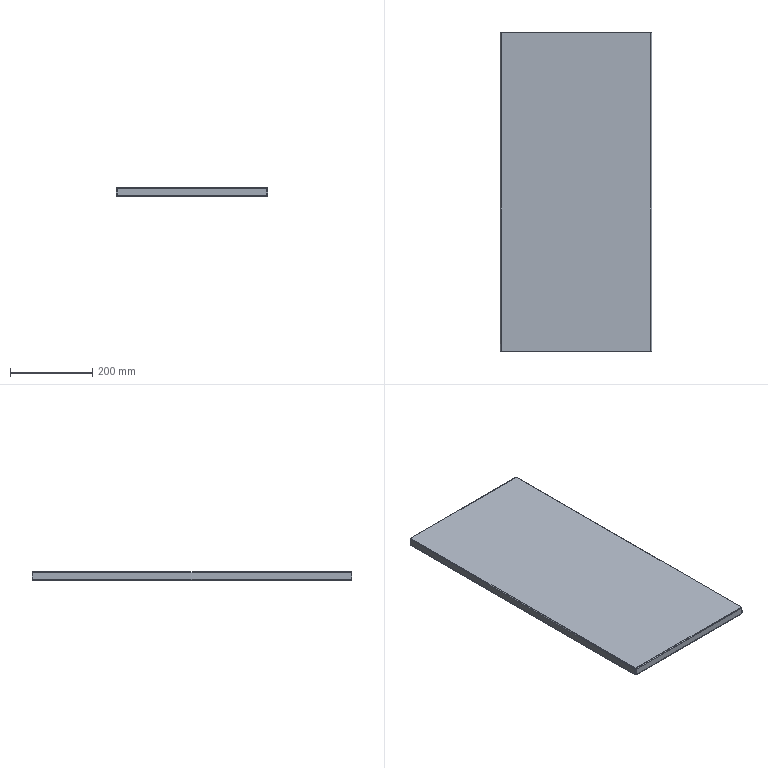Part | STEP file | X77-03008 | 1 solid | 70 faces | box 368 x 778 x 20 mm | volume 516743 mm3 | plane 38 | spline 16 | cylinder 16 | commonest cylinder face diameters 1.473 x8 4.473 x8